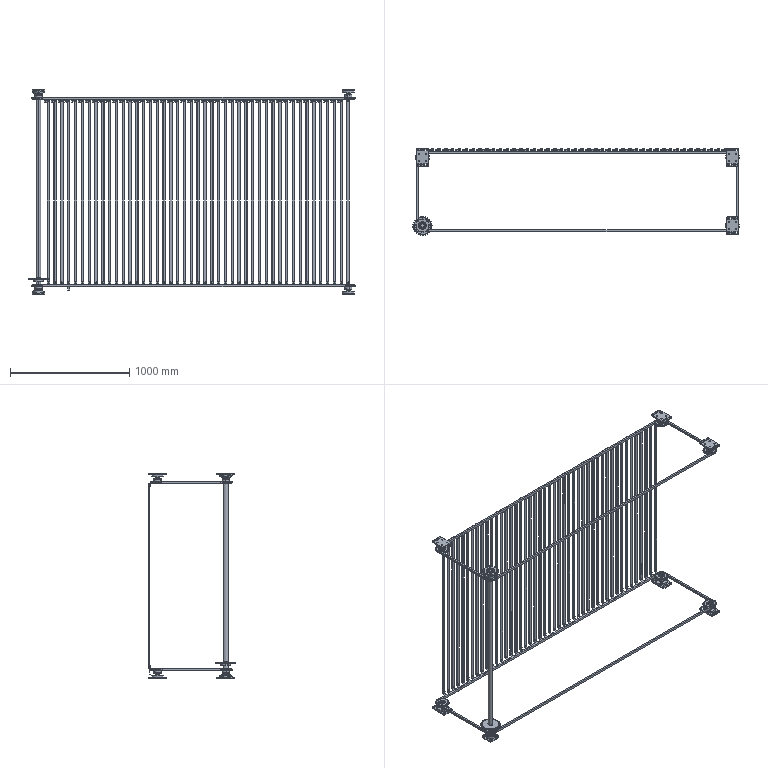Part | SolidWorks | features ReferencePattern 44, CompositeCurve 1, LocalLPattern 1 | 94 solids | 5023 faces | volume 13271643 mm3 | cylinder 1820 | plane 1601 | torus 776 | sphere 408 | spline 352 | cone 66 | commonest cylinder face diameters 55.039 x280 12.191 x218 4.2 x180 5.5 x180 10 x180 115.416 x136